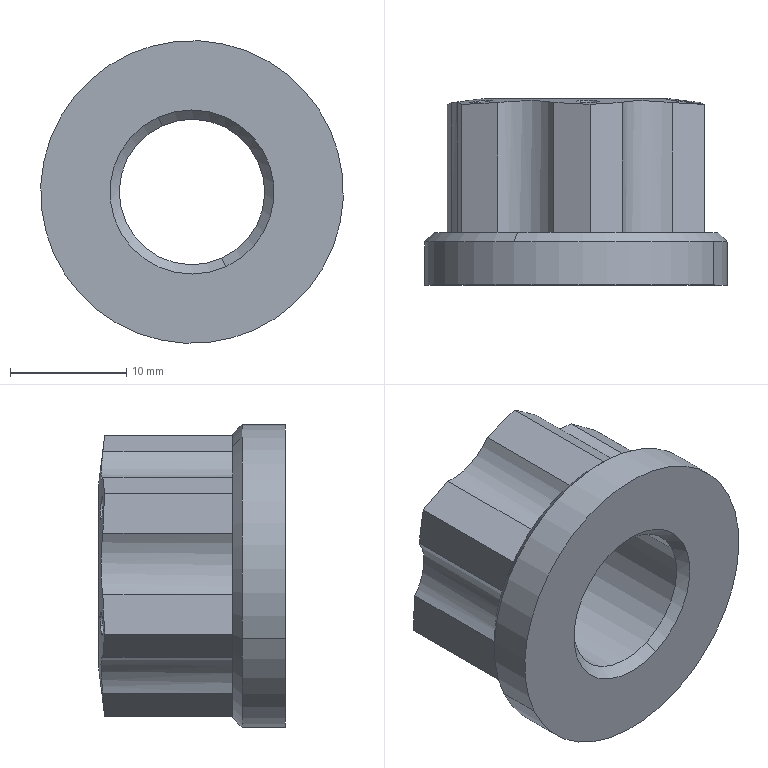Part | SolidWorks | features BaseBody 1 | 1 solid | 51 faces | box 26 x 16 x 26 mm | volume 4470 mm3 | cylinder 22 | plane 15 | cone 8 | sphere 6 | commonest cylinder face diameters 2 x12 8 x6 12.5 x2 26 x2